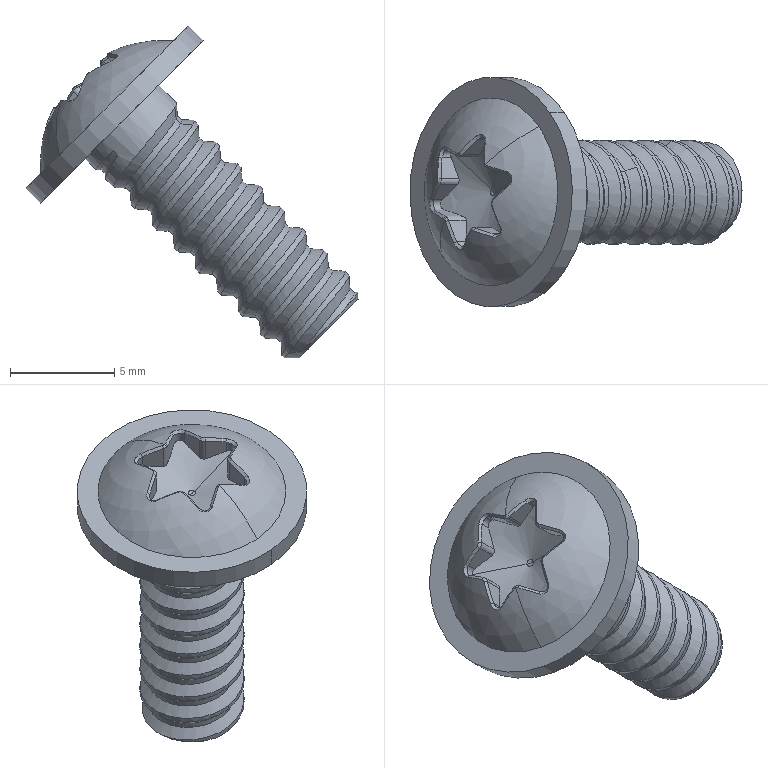Part | SolidWorks | features BaseBody 1 | 1 solid | 95 faces | box 15.91 x 11 x 15.91 mm | volume 379.281 mm3 | cylinder 33 | spline 26 | cone 17 | plane 15 | sphere 4 | commonest cylinder face diameters 5 x19 0.6 x12 11 x2